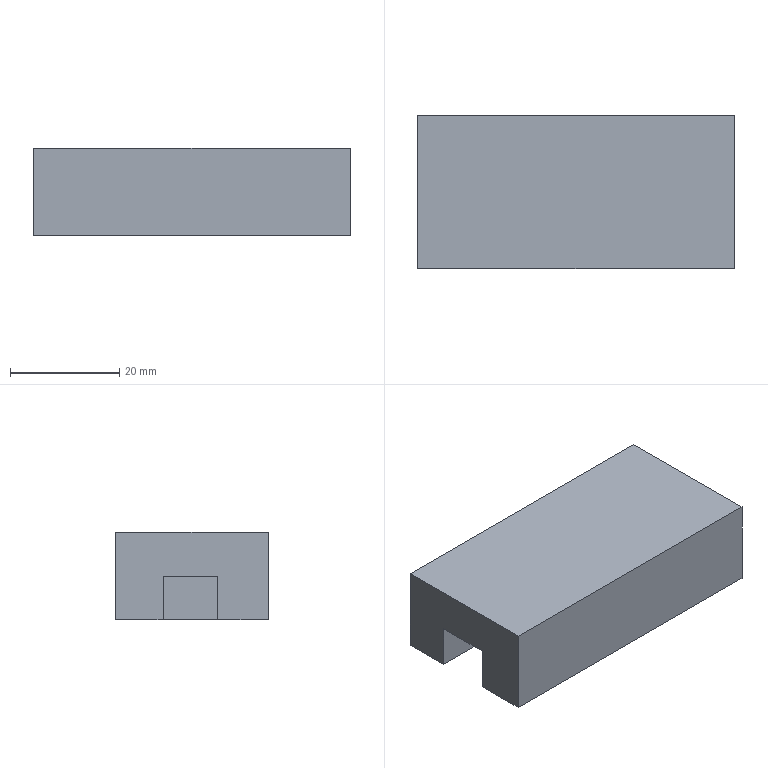Part | STEP file | 手指夹-2 | 1 solid | 10 faces | box 58 x 28 x 16 mm | volume 24327 mm3 | plane 10
STEP:
#1=CARTESIAN_POINT('',(2.556,-14.301,8.));
#2=VERTEX_POINT('',#1);
#3=CARTESIAN_POINT('',(2.556,-14.301,-8.));
#4=VERTEX_POINT('',#3);
#5=CARTESIAN_POINT('',(2.556,-14.301,8.));
#6=DIRECTION('',(0.,0.,-1.));
#7=VECTOR('',#6,1000.);
#8=LINE('',#5,#7);
#9=EDGE_CURVE('',#2,#4,#8,.T.);
#10=ORIENTED_EDGE('',*,*,#9,.T.);
#11=CARTESIAN_POINT('',(60.556,-14.301,-8.));
#12=VERTEX_POINT('',#11);
#13=CARTESIAN_POINT('',(2.556,-14.301,-8.));
#14=DIRECTION('',(-1.,0.,0.));
#15=VECTOR('',#14,1000.);
#16=LINE('',#13,#15);
#17=EDGE_CURVE('',#12,#4,#16,.T.);
#18=ORIENTED_EDGE('',*,*,#17,.F.);
#19=CARTESIAN_POINT('',(60.556,-14.301,8.));
#20=VERTEX_POINT('',#19);
#21=CARTESIAN_POINT('',(60.556,-14.301,8.));
#22=DIRECTION('',(0.,0.,-1.));
#23=VECTOR('',#22,1000.);
#24=LINE('',#21,#23);
#25=EDGE_CURVE('',#20,#12,#24,.T.);
#26=ORIENTED_EDGE('',*,*,#25,.F.);
#27=CARTESIAN_POINT('',(2.556,-14.301,8.));
#28=DIRECTION('',(1.,0.,0.));
#29=VECTOR('',#28,1000.);
#30=LINE('',#27,#29);
#31=EDGE_CURVE('',#2,#20,#30,.T.);
#32=ORIENTED_EDGE('',*,*,#31,.F.);
#33=EDGE_LOOP('',(#10,#18,#26,#32));
#34=FACE_OUTER_BOUND('',#33,.T.);
#35=CARTESIAN_POINT('',(2.556,-14.301,8.));
#36=DIRECTION('',(0.,1.,0.));
#37=DIRECTION('',(-1.,0.,0.));
#38=AXIS2_PLACEMENT_3D('',#35,#36,#37);
#39=PLANE('',#38);
#40=ADVANCED_FACE('',(#34),#39,.F.);
#41=ORIENTED_EDGE('',*,*,#25,.T.);
#42=CARTESIAN_POINT('',(60.556,13.699,-8.));
#43=VERTEX_POINT('',#42);
#44=CARTESIAN_POINT('',(60.556,13.699,-8.));
#45=DIRECTION('',(0.,-1.,0.));
#46=VECTOR('',#45,1000.);
#47=LINE('',#44,#46);
#48=EDGE_CURVE('',#43,#12,#47,.T.);
#49=ORIENTED_EDGE('',*,*,#48,.F.);
#50=CARTESIAN_POINT('',(60.556,13.699,8.));
#51=VERTEX_POINT('',#50);
#52=CARTESIAN_POINT('',(60.556,13.699,8.));
#53=DIRECTION('',(0.,0.,-1.));
#54=VECTOR('',#53,1000.);
#55=LINE('',#52,#54);
#56=EDGE_CURVE('',#51,#43,#55,.T.);
#57=ORIENTED_EDGE('',*,*,#56,.F.);
#58=CARTESIAN_POINT('',(60.556,13.699,8.));
#59=DIRECTION('',(0.,1.,0.));
#60=VECTOR('',#59,1000.);
#61=LINE('',#58,#60);
#62=EDGE_CURVE('',#20,#51,#61,.T.);
#63=ORIENTED_EDGE('',*,*,#62,.F.);
#64=EDGE_LOOP('',(#41,#49,#57,#63));
#65=FACE_OUTER_BOUND('',#64,.T.);
#66=CARTESIAN_POINT('',(60.556,13.699,8.));
#67=DIRECTION('',(-1.,0.,0.));
#68=DIRECTION('',(0.,-1.,0.));
#69=AXIS2_PLACEMENT_3D('',#66,#67,#68);
#70=PLANE('',#69);
#71=ADVANCED_FACE('',(#65),#70,.F.);
#72=ORIENTED_EDGE('',*,*,#56,.T.);
#73=CARTESIAN_POINT('',(2.556,13.699,-8.));
#74=VERTEX_POINT('',#73);
#75=CARTESIAN_POINT('',(2.556,13.699,-8.));
#76=DIRECTION('',(1.,0.,0.));
#77=VECTOR('',#76,1000.);
#78=LINE('',#75,#77);
#79=EDGE_CURVE('',#74,#43,#78,.T.);
#80=ORIENTED_EDGE('',*,*,#79,.F.);
#81=CARTESIAN_POINT('',(2.556,13.699,8.));
#82=VERTEX_POINT('',#81);
#83=CARTESIAN_POINT('',(2.556,13.699,8.));
#84=DIRECTION('',(0.,0.,-1.));
#85=VECTOR('',#84,1000.);
#86=LINE('',#83,#85);
#87=EDGE_CURVE('',#82,#74,#86,.T.);
#88=ORIENTED_EDGE('',*,*,#87,.F.);
#89=CARTESIAN_POINT('',(2.556,13.699,8.));
#90=DIRECTION('',(-1.,0.,0.));
#91=VECTOR('',#90,1000.);
#92=LINE('',#89,#91);
#93=EDGE_CURVE('',#51,#82,#92,.T.);
#94=ORIENTED_EDGE('',*,*,#93,.F.);
#95=EDGE_LOOP('',(#72,#80,#88,#94));
#96=FACE_OUTER_BOUND('',#95,.T.);
#97=CARTESIAN_POINT('',(2.556,13.699,8.));
#98=DIRECTION('',(0.,-1.,0.));
#99=DIRECTION('',(1.,0.,0.));
#100=AXIS2_PLACEMENT_3D('',#97,#98,#99);
#101=PLANE('',#100);
#102=ADVANCED_FACE('',(#96),#101,.F.);
#103=ORIENTED_EDGE('',*,*,#87,.T.);
#104=CARTESIAN_POINT('',(2.556,5.,-8.));
#105=VERTEX_POINT('',#104);
#106=CARTESIAN_POINT('',(2.556,13.699,-8.));
#107=DIRECTION('',(0.,1.,0.));
#108=VECTOR('',#107,1000.);
#109=LINE('',#106,#108);
#110=EDGE_CURVE('',#105,#74,#109,.T.);
#111=ORIENTED_EDGE('',*,*,#110,.F.);
#112=CARTESIAN_POINT('',(2.556,5.,0.));
#113=VERTEX_POINT('',#112);
#114=CARTESIAN_POINT('',(2.556,5.,-8.));
#115=DIRECTION('',(0.,0.,1.));
#116=VECTOR('',#115,1000.);
#117=LINE('',#114,#116);
#118=EDGE_CURVE('',#105,#113,#117,.T.);
#119=ORIENTED_EDGE('',*,*,#118,.T.);
#120=CARTESIAN_POINT('',(2.556,-5.,0.));
#121=VERTEX_POINT('',#120);
#122=CARTESIAN_POINT('',(2.556,13.699,0.));
#123=DIRECTION('',(0.,-1.,0.));
#124=VECTOR('',#123,1000.);
#125=LINE('',#122,#124);
#126=EDGE_CURVE('',#113,#121,#125,.T.);
#127=ORIENTED_EDGE('',*,*,#126,.T.);
#128=CARTESIAN_POINT('',(2.556,-5.,-8.));
#129=VERTEX_POINT('',#128);
#130=CARTESIAN_POINT('',(2.556,-5.,-8.));
#131=DIRECTION('',(0.,0.,1.));
#132=VECTOR('',#131,1000.);
#133=LINE('',#130,#132);
#134=EDGE_CURVE('',#129,#121,#133,.T.);
#135=ORIENTED_EDGE('',*,*,#134,.F.);
#136=CARTESIAN_POINT('',(2.556,-5.,-8.));
#137=DIRECTION('',(0.,1.,0.));
#138=VECTOR('',#137,1000.);
#139=LINE('',#136,#138);
#140=EDGE_CURVE('',#4,#129,#139,.T.);
#141=ORIENTED_EDGE('',*,*,#140,.F.);
#142=ORIENTED_EDGE('',*,*,#9,.F.);
#143=CARTESIAN_POINT('',(2.556,13.699,8.));
#144=DIRECTION('',(0.,-1.,0.));
#145=VECTOR('',#144,1000.);
#146=LINE('',#143,#145);
#147=EDGE_CURVE('',#82,#2,#146,.T.);
#148=ORIENTED_EDGE('',*,*,#147,.F.);
#149=EDGE_LOOP('',(#103,#111,#119,#127,#135,#141,#142,#148));
#150=FACE_OUTER_BOUND('',#149,.T.);
#151=CARTESIAN_POINT('',(2.556,13.699,8.));
#152=DIRECTION('',(1.,0.,0.));
#153=DIRECTION('',(0.,1.,0.));
#154=AXIS2_PLACEMENT_3D('',#151,#152,#153);
#155=PLANE('',#154);
#156=ADVANCED_FACE('',(#150),#155,.F.);
#157=ORIENTED_EDGE('',*,*,#31,.T.);
#158=ORIENTED_EDGE('',*,*,#62,.T.);
#159=ORIENTED_EDGE('',*,*,#93,.T.);
#160=ORIENTED_EDGE('',*,*,#147,.T.);
#161=EDGE_LOOP('',(#157,#158,#159,#160));
#162=FACE_OUTER_BOUND('',#161,.T.);
#163=CARTESIAN_POINT('',(60.556,-14.301,8.));
#164=DIRECTION('',(0.,0.,-1.));
#165=DIRECTION('',(-1.,0.,0.));
#166=AXIS2_PLACEMENT_3D('',#163,#164,#165);
#167=PLANE('',#166);
#168=ADVANCED_FACE('',(#162),#167,.F.);
#169=CARTESIAN_POINT('',(23.269,5.,0.));
#170=VERTEX_POINT('',#169);
#171=CARTESIAN_POINT('',(2.556,5.,0.));
#172=DIRECTION('',(-1.,0.,0.));
#173=VECTOR('',#172,1000.);
#174=LINE('',#171,#173);
#175=EDGE_CURVE('',#170,#113,#174,.T.);
#176=ORIENTED_EDGE('',*,*,#175,.F.);
#177=CARTESIAN_POINT('',(23.269,-5.,0.));
#178=VERTEX_POINT('',#177);
#179=CARTESIAN_POINT('',(23.269,5.,0.));
#180=DIRECTION('',(0.,1.,0.));
#181=VECTOR('',#180,1000.);
#182=LINE('',#179,#181);
#183=EDGE_CURVE('',#178,#170,#182,.T.);
#184=ORIENTED_EDGE('',*,*,#183,.F.);
#185=CARTESIAN_POINT('',(2.556,-5.,0.));
#186=DIRECTION('',(1.,0.,0.));
#187=VECTOR('',#186,1000.);
#188=LINE('',#185,#187);
#189=EDGE_CURVE('',#121,#178,#188,.T.);
#190=ORIENTED_EDGE('',*,*,#189,.F.);
#191=ORIENTED_EDGE('',*,*,#126,.F.);
#192=EDGE_LOOP('',(#176,#184,#190,#191));
#193=FACE_OUTER_BOUND('',#192,.T.);
#194=CARTESIAN_POINT('',(60.556,-14.301,0.));
#195=DIRECTION('',(0.,0.,-1.));
#196=DIRECTION('',(-1.,0.,0.));
#197=AXIS2_PLACEMENT_3D('',#194,#195,#196);
#198=PLANE('',#197);
#199=ADVANCED_FACE('',(#193),#198,.T.);
#200=ORIENTED_EDGE('',*,*,#189,.T.);
#201=CARTESIAN_POINT('',(23.269,-5.,-8.));
#202=VERTEX_POINT('',#201);
#203=CARTESIAN_POINT('',(23.269,-5.,-8.));
#204=DIRECTION('',(0.,0.,1.));
#205=VECTOR('',#204,1000.);
#206=LINE('',#203,#205);
#207=EDGE_CURVE('',#202,#178,#206,.T.);
#208=ORIENTED_EDGE('',*,*,#207,.F.);
#209=CARTESIAN_POINT('',(2.556,-5.,-8.));
#210=DIRECTION('',(1.,0.,0.));
#211=VECTOR('',#210,1000.);
#212=LINE('',#209,#211);
#213=EDGE_CURVE('',#129,#202,#212,.T.);
#214=ORIENTED_EDGE('',*,*,#213,.F.);
#215=ORIENTED_EDGE('',*,*,#134,.T.);
#216=EDGE_LOOP('',(#200,#208,#214,#215));
#217=FACE_OUTER_BOUND('',#216,.T.);
#218=CARTESIAN_POINT('',(2.556,-5.,-8.));
#219=DIRECTION('',(0.,-1.,0.));
#220=DIRECTION('',(1.,0.,0.));
#221=AXIS2_PLACEMENT_3D('',#218,#219,#220);
#222=PLANE('',#221);
#223=ADVANCED_FACE('',(#217),#222,.F.);
#224=ORIENTED_EDGE('',*,*,#183,.T.);
#225=CARTESIAN_POINT('',(23.269,5.,-8.));
#226=VERTEX_POINT('',#225);
#227=CARTESIAN_POINT('',(23.269,5.,-8.));
#228=DIRECTION('',(0.,0.,1.));
#229=VECTOR('',#228,1000.);
#230=LINE('',#227,#229);
#231=EDGE_CURVE('',#226,#170,#230,.T.);
#232=ORIENTED_EDGE('',*,*,#231,.F.);
#233=CARTESIAN_POINT('',(23.269,5.,-8.));
#234=DIRECTION('',(0.,1.,0.));
#235=VECTOR('',#234,1000.);
#236=LINE('',#233,#235);
#237=EDGE_CURVE('',#202,#226,#236,.T.);
#238=ORIENTED_EDGE('',*,*,#237,.F.);
#239=ORIENTED_EDGE('',*,*,#207,.T.);
#240=EDGE_LOOP('',(#224,#232,#238,#239));
#241=FACE_OUTER_BOUND('',#240,.T.);
#242=CARTESIAN_POINT('',(23.269,5.,-8.));
#243=DIRECTION('',(1.,0.,0.));
#244=DIRECTION('',(0.,0.,-1.));
#245=AXIS2_PLACEMENT_3D('',#242,#243,#244);
#246=PLANE('',#245);
#247=ADVANCED_FACE('',(#241),#246,.F.);
#248=ORIENTED_EDGE('',*,*,#175,.T.);
#249=ORIENTED_EDGE('',*,*,#118,.F.);
#250=CARTESIAN_POINT('',(2.556,5.,-8.));
#251=DIRECTION('',(-1.,0.,0.));
#252=VECTOR('',#251,1000.);
#253=LINE('',#250,#252);
#254=EDGE_CURVE('',#226,#105,#253,.T.);
#255=ORIENTED_EDGE('',*,*,#254,.F.);
#256=ORIENTED_EDGE('',*,*,#231,.T.);
#257=EDGE_LOOP('',(#248,#249,#255,#256));
#258=FACE_OUTER_BOUND('',#257,.T.);
#259=CARTESIAN_POINT('',(2.556,5.,-8.));
#260=DIRECTION('',(0.,1.,0.));
#261=DIRECTION('',(0.,0.,1.));
#262=AXIS2_PLACEMENT_3D('',#259,#260,#261);
#263=PLANE('',#262);
#264=ADVANCED_FACE('',(#258),#263,.F.);
#265=ORIENTED_EDGE('',*,*,#110,.T.);
#266=ORIENTED_EDGE('',*,*,#79,.T.);
#267=ORIENTED_EDGE('',*,*,#48,.T.);
#268=ORIENTED_EDGE('',*,*,#17,.T.);
#269=ORIENTED_EDGE('',*,*,#140,.T.);
#270=ORIENTED_EDGE('',*,*,#213,.T.);
#271=ORIENTED_EDGE('',*,*,#237,.T.);
#272=ORIENTED_EDGE('',*,*,#254,.T.);
#273=EDGE_LOOP('',(#265,#266,#267,#268,#269,#270,#271,#272));
#274=FACE_OUTER_BOUND('',#273,.T.);
#275=CARTESIAN_POINT('',(2.556,5.,-8.));
#276=DIRECTION('',(0.,0.,1.));
#277=DIRECTION('',(1.,0.,0.));
#278=AXIS2_PLACEMENT_3D('',#275,#276,#277);
#279=PLANE('',#278);
#280=ADVANCED_FACE('',(#274),#279,.F.);
#281=CLOSED_SHELL('',(#40,#71,#102,#156,#168,#199,#223,#247,#264,#280));
#282=MANIFOLD_SOLID_BREP('',#281);
#283=CARTESIAN_POINT('',(0.,0.,0.));
#284=DIRECTION('',(0.,0.,1.));
#285=DIRECTION('',(1.,0.,0.));
#286=AXIS2_PLACEMENT_3D('',#283,#284,#285);
#287=(LENGTH_UNIT()NAMED_UNIT(*)SI_UNIT(.MILLI.,.METRE.));
#288=UNCERTAINTY_MEASURE_WITH_UNIT(LENGTH_MEASURE(0.00001),#287,'','');
#289=(NAMED_UNIT(*)PLANE_ANGLE_UNIT()SI_UNIT($,.RADIAN.));
#290=(NAMED_UNIT(*)SI_UNIT($,.STERADIAN.)SOLID_ANGLE_UNIT());
#291=(GEOMETRIC_REPRESENTATION_CONTEXT(3)GLOBAL_UNCERTAINTY_ASSIGNED_CONTEXT((#288))GLOBAL_UNIT_ASSIGNED_CONTEXT((#287,#289,#290))REPRESENTATION_CONTEXT('',''));
#292=ADVANCED_BREP_SHAPE_REPRESENTATION('',(#282,#286),#291);